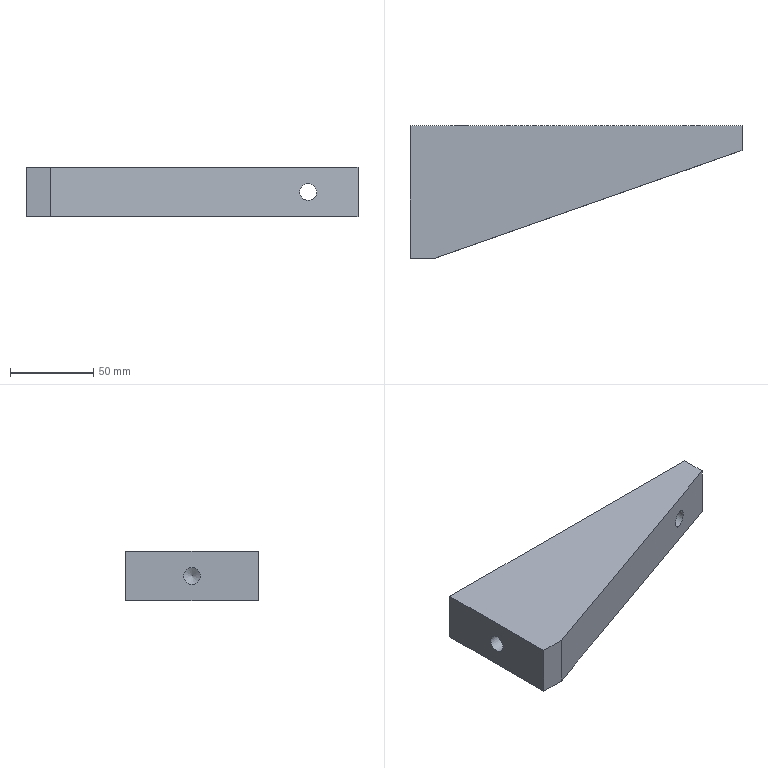Part | NX | features stifener2 2 | 1 solid | 12 faces | volume 292583 mm3 | plane 7 | cylinder 3 | cone 2 | commonest cylinder face diameters 10.2 x3